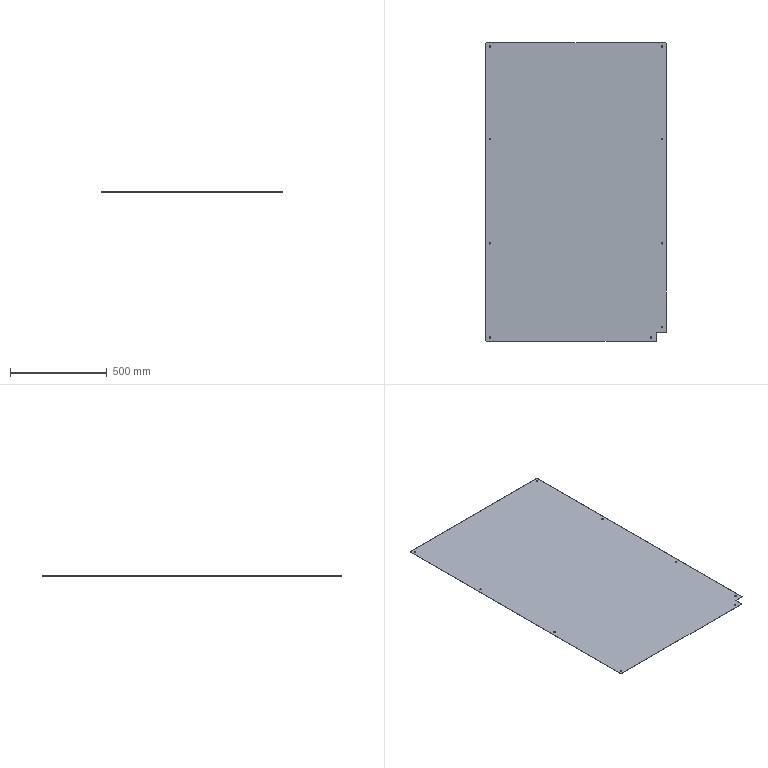Part | SolidWorks | features ICE 5, Fillet 2, FlatPattern 1, HoleWzd 1, SMBaseFlange 1, SheetMetal 1 | 1 solid | 32 faces | box 933 x 1548 x 1.2 mm | volume 1730124 mm3 | cylinder 24 | plane 8 | commonest cylinder face diameters 7 x18 6 x6
STEP:
#1=CARTESIAN_POINT('',(16.5,-20.,0.));
#2=VERTEX_POINT('',#1);
#3=CARTESIAN_POINT('',(23.5,-20.,0.));
#4=VERTEX_POINT('',#3);
#5=CARTESIAN_POINT('',(20.,-20.,0.));
#6=DIRECTION('',(0.,0.,1.));
#7=DIRECTION('',(1.,0.,0.));
#8=AXIS2_PLACEMENT_3D('',#5,#6,#7);
#9=CIRCLE('',#8,3.5);
#10=EDGE_CURVE('',#2,#4,#9,.T.);
#11=ORIENTED_EDGE('',*,*,#10,.F.);
#12=CARTESIAN_POINT('',(16.5,-20.,1.2));
#13=VERTEX_POINT('',#12);
#14=CARTESIAN_POINT('',(16.5,-20.,1.2));
#15=DIRECTION('',(0.,0.,1.));
#16=VECTOR('',#15,1000.);
#17=LINE('',#14,#16);
#18=EDGE_CURVE('',#2,#13,#17,.T.);
#19=ORIENTED_EDGE('',*,*,#18,.T.);
#20=CARTESIAN_POINT('',(23.5,-20.,1.2));
#21=VERTEX_POINT('',#20);
#22=CARTESIAN_POINT('',(20.,-20.,1.2));
#23=DIRECTION('',(0.,0.,1.));
#24=DIRECTION('',(1.,0.,0.));
#25=AXIS2_PLACEMENT_3D('',#22,#23,#24);
#26=CIRCLE('',#25,3.5);
#27=EDGE_CURVE('',#13,#21,#26,.T.);
#28=ORIENTED_EDGE('',*,*,#27,.T.);
#29=CARTESIAN_POINT('',(23.5,-20.,1.2));
#30=DIRECTION('',(0.,0.,1.));
#31=VECTOR('',#30,1000.);
#32=LINE('',#29,#31);
#33=EDGE_CURVE('',#4,#21,#32,.T.);
#34=ORIENTED_EDGE('',*,*,#33,.F.);
#35=EDGE_LOOP('',(#11,#19,#28,#34));
#36=FACE_OUTER_BOUND('',#35,.T.);
#37=CARTESIAN_POINT('',(20.,-20.,1.2));
#38=DIRECTION('',(0.,0.,1.));
#39=DIRECTION('',(1.,0.,0.));
#40=AXIS2_PLACEMENT_3D('',#37,#38,#39);
#41=CYLINDRICAL_SURFACE('',#40,3.5);
#42=ADVANCED_FACE('',(#36),#41,.F.);
#43=CARTESIAN_POINT('',(909.5,-20.,0.));
#44=VERTEX_POINT('',#43);
#45=CARTESIAN_POINT('',(916.5,-20.,0.));
#46=VERTEX_POINT('',#45);
#47=CARTESIAN_POINT('',(913.,-20.,0.));
#48=DIRECTION('',(0.,0.,1.));
#49=DIRECTION('',(1.,0.,0.));
#50=AXIS2_PLACEMENT_3D('',#47,#48,#49);
#51=CIRCLE('',#50,3.5);
#52=EDGE_CURVE('',#44,#46,#51,.T.);
#53=ORIENTED_EDGE('',*,*,#52,.F.);
#54=CARTESIAN_POINT('',(909.5,-20.,1.2));
#55=VERTEX_POINT('',#54);
#56=CARTESIAN_POINT('',(909.5,-20.,1.2));
#57=DIRECTION('',(0.,0.,1.));
#58=VECTOR('',#57,1000.);
#59=LINE('',#56,#58);
#60=EDGE_CURVE('',#44,#55,#59,.T.);
#61=ORIENTED_EDGE('',*,*,#60,.T.);
#62=CARTESIAN_POINT('',(916.5,-20.,1.2));
#63=VERTEX_POINT('',#62);
#64=CARTESIAN_POINT('',(913.,-20.,1.2));
#65=DIRECTION('',(0.,0.,1.));
#66=DIRECTION('',(1.,0.,0.));
#67=AXIS2_PLACEMENT_3D('',#64,#65,#66);
#68=CIRCLE('',#67,3.5);
#69=EDGE_CURVE('',#55,#63,#68,.T.);
#70=ORIENTED_EDGE('',*,*,#69,.T.);
#71=CARTESIAN_POINT('',(916.5,-20.,1.2));
#72=DIRECTION('',(0.,0.,1.));
#73=VECTOR('',#72,1000.);
#74=LINE('',#71,#73);
#75=EDGE_CURVE('',#46,#63,#74,.T.);
#76=ORIENTED_EDGE('',*,*,#75,.F.);
#77=EDGE_LOOP('',(#53,#61,#70,#76));
#78=FACE_OUTER_BOUND('',#77,.T.);
#79=CARTESIAN_POINT('',(913.,-20.,1.2));
#80=DIRECTION('',(0.,0.,1.));
#81=DIRECTION('',(1.,0.,0.));
#82=AXIS2_PLACEMENT_3D('',#79,#80,#81);
#83=CYLINDRICAL_SURFACE('',#82,3.5);
#84=ADVANCED_FACE('',(#78),#83,.F.);
#85=CARTESIAN_POINT('',(16.5,-1528.,0.));
#86=VERTEX_POINT('',#85);
#87=CARTESIAN_POINT('',(23.5,-1528.,0.));
#88=VERTEX_POINT('',#87);
#89=CARTESIAN_POINT('',(20.,-1528.,0.));
#90=DIRECTION('',(0.,0.,1.));
#91=DIRECTION('',(1.,0.,0.));
#92=AXIS2_PLACEMENT_3D('',#89,#90,#91);
#93=CIRCLE('',#92,3.5);
#94=EDGE_CURVE('',#86,#88,#93,.T.);
#95=ORIENTED_EDGE('',*,*,#94,.F.);
#96=CARTESIAN_POINT('',(16.5,-1528.,1.2));
#97=VERTEX_POINT('',#96);
#98=CARTESIAN_POINT('',(16.5,-1528.,1.2));
#99=DIRECTION('',(0.,0.,1.));
#100=VECTOR('',#99,1000.);
#101=LINE('',#98,#100);
#102=EDGE_CURVE('',#86,#97,#101,.T.);
#103=ORIENTED_EDGE('',*,*,#102,.T.);
#104=CARTESIAN_POINT('',(23.5,-1528.,1.2));
#105=VERTEX_POINT('',#104);
#106=CARTESIAN_POINT('',(20.,-1528.,1.2));
#107=DIRECTION('',(0.,0.,1.));
#108=DIRECTION('',(1.,0.,0.));
#109=AXIS2_PLACEMENT_3D('',#106,#107,#108);
#110=CIRCLE('',#109,3.5);
#111=EDGE_CURVE('',#97,#105,#110,.T.);
#112=ORIENTED_EDGE('',*,*,#111,.T.);
#113=CARTESIAN_POINT('',(23.5,-1528.,1.2));
#114=DIRECTION('',(0.,0.,1.));
#115=VECTOR('',#114,1000.);
#116=LINE('',#113,#115);
#117=EDGE_CURVE('',#88,#105,#116,.T.);
#118=ORIENTED_EDGE('',*,*,#117,.F.);
#119=EDGE_LOOP('',(#95,#103,#112,#118));
#120=FACE_OUTER_BOUND('',#119,.T.);
#121=CARTESIAN_POINT('',(20.,-1528.,1.2));
#122=DIRECTION('',(0.,0.,1.));
#123=DIRECTION('',(1.,0.,0.));
#124=AXIS2_PLACEMENT_3D('',#121,#122,#123);
#125=CYLINDRICAL_SURFACE('',#124,3.5);
#126=ADVANCED_FACE('',(#120),#125,.F.);
#127=CARTESIAN_POINT('',(851.5,-1528.,0.));
#128=VERTEX_POINT('',#127);
#129=CARTESIAN_POINT('',(858.5,-1528.,0.));
#130=VERTEX_POINT('',#129);
#131=CARTESIAN_POINT('',(855.,-1528.,0.));
#132=DIRECTION('',(0.,0.,1.));
#133=DIRECTION('',(1.,0.,0.));
#134=AXIS2_PLACEMENT_3D('',#131,#132,#133);
#135=CIRCLE('',#134,3.5);
#136=EDGE_CURVE('',#128,#130,#135,.T.);
#137=ORIENTED_EDGE('',*,*,#136,.F.);
#138=CARTESIAN_POINT('',(851.5,-1528.,1.2));
#139=VERTEX_POINT('',#138);
#140=CARTESIAN_POINT('',(851.5,-1528.,1.2));
#141=DIRECTION('',(0.,0.,1.));
#142=VECTOR('',#141,1000.);
#143=LINE('',#140,#142);
#144=EDGE_CURVE('',#128,#139,#143,.T.);
#145=ORIENTED_EDGE('',*,*,#144,.T.);
#146=CARTESIAN_POINT('',(858.5,-1528.,1.2));
#147=VERTEX_POINT('',#146);
#148=CARTESIAN_POINT('',(855.,-1528.,1.2));
#149=DIRECTION('',(0.,0.,1.));
#150=DIRECTION('',(1.,0.,0.));
#151=AXIS2_PLACEMENT_3D('',#148,#149,#150);
#152=CIRCLE('',#151,3.5);
#153=EDGE_CURVE('',#139,#147,#152,.T.);
#154=ORIENTED_EDGE('',*,*,#153,.T.);
#155=CARTESIAN_POINT('',(858.5,-1528.,1.2));
#156=DIRECTION('',(0.,0.,1.));
#157=VECTOR('',#156,1000.);
#158=LINE('',#155,#157);
#159=EDGE_CURVE('',#130,#147,#158,.T.);
#160=ORIENTED_EDGE('',*,*,#159,.F.);
#161=EDGE_LOOP('',(#137,#145,#154,#160));
#162=FACE_OUTER_BOUND('',#161,.T.);
#163=CARTESIAN_POINT('',(855.,-1528.,1.2));
#164=DIRECTION('',(0.,0.,1.));
#165=DIRECTION('',(1.,0.,0.));
#166=AXIS2_PLACEMENT_3D('',#163,#164,#165);
#167=CYLINDRICAL_SURFACE('',#166,3.5);
#168=ADVANCED_FACE('',(#162),#167,.F.);
#169=CARTESIAN_POINT('',(16.5,-1040.,0.));
#170=VERTEX_POINT('',#169);
#171=CARTESIAN_POINT('',(23.5,-1040.,0.));
#172=VERTEX_POINT('',#171);
#173=CARTESIAN_POINT('',(20.,-1040.,0.));
#174=DIRECTION('',(0.,0.,1.));
#175=DIRECTION('',(1.,0.,0.));
#176=AXIS2_PLACEMENT_3D('',#173,#174,#175);
#177=CIRCLE('',#176,3.5);
#178=EDGE_CURVE('',#170,#172,#177,.T.);
#179=ORIENTED_EDGE('',*,*,#178,.F.);
#180=CARTESIAN_POINT('',(16.5,-1040.,1.2));
#181=VERTEX_POINT('',#180);
#182=CARTESIAN_POINT('',(16.5,-1040.,1.2));
#183=DIRECTION('',(0.,0.,1.));
#184=VECTOR('',#183,1000.);
#185=LINE('',#182,#184);
#186=EDGE_CURVE('',#170,#181,#185,.T.);
#187=ORIENTED_EDGE('',*,*,#186,.T.);
#188=CARTESIAN_POINT('',(23.5,-1040.,1.2));
#189=VERTEX_POINT('',#188);
#190=CARTESIAN_POINT('',(20.,-1040.,1.2));
#191=DIRECTION('',(0.,0.,1.));
#192=DIRECTION('',(1.,0.,0.));
#193=AXIS2_PLACEMENT_3D('',#190,#191,#192);
#194=CIRCLE('',#193,3.5);
#195=EDGE_CURVE('',#181,#189,#194,.T.);
#196=ORIENTED_EDGE('',*,*,#195,.T.);
#197=CARTESIAN_POINT('',(23.5,-1040.,1.2));
#198=DIRECTION('',(0.,0.,1.));
#199=VECTOR('',#198,1000.);
#200=LINE('',#197,#199);
#201=EDGE_CURVE('',#172,#189,#200,.T.);
#202=ORIENTED_EDGE('',*,*,#201,.F.);
#203=EDGE_LOOP('',(#179,#187,#196,#202));
#204=FACE_OUTER_BOUND('',#203,.T.);
#205=CARTESIAN_POINT('',(20.,-1040.,1.2));
#206=DIRECTION('',(0.,0.,1.));
#207=DIRECTION('',(1.,0.,0.));
#208=AXIS2_PLACEMENT_3D('',#205,#206,#207);
#209=CYLINDRICAL_SURFACE('',#208,3.5);
#210=ADVANCED_FACE('',(#204),#209,.F.);
#211=CARTESIAN_POINT('',(909.5,-1040.,0.));
#212=VERTEX_POINT('',#211);
#213=CARTESIAN_POINT('',(916.5,-1040.,0.));
#214=VERTEX_POINT('',#213);
#215=CARTESIAN_POINT('',(913.,-1040.,0.));
#216=DIRECTION('',(0.,0.,1.));
#217=DIRECTION('',(1.,0.,0.));
#218=AXIS2_PLACEMENT_3D('',#215,#216,#217);
#219=CIRCLE('',#218,3.5);
#220=EDGE_CURVE('',#212,#214,#219,.T.);
#221=ORIENTED_EDGE('',*,*,#220,.F.);
#222=CARTESIAN_POINT('',(909.5,-1040.,1.2));
#223=VERTEX_POINT('',#222);
#224=CARTESIAN_POINT('',(909.5,-1040.,1.2));
#225=DIRECTION('',(0.,0.,1.));
#226=VECTOR('',#225,1000.);
#227=LINE('',#224,#226);
#228=EDGE_CURVE('',#212,#223,#227,.T.);
#229=ORIENTED_EDGE('',*,*,#228,.T.);
#230=CARTESIAN_POINT('',(916.5,-1040.,1.2));
#231=VERTEX_POINT('',#230);
#232=CARTESIAN_POINT('',(913.,-1040.,1.2));
#233=DIRECTION('',(0.,0.,1.));
#234=DIRECTION('',(1.,0.,0.));
#235=AXIS2_PLACEMENT_3D('',#232,#233,#234);
#236=CIRCLE('',#235,3.5);
#237=EDGE_CURVE('',#223,#231,#236,.T.);
#238=ORIENTED_EDGE('',*,*,#237,.T.);
#239=CARTESIAN_POINT('',(916.5,-1040.,1.2));
#240=DIRECTION('',(0.,0.,1.));
#241=VECTOR('',#240,1000.);
#242=LINE('',#239,#241);
#243=EDGE_CURVE('',#214,#231,#242,.T.);
#244=ORIENTED_EDGE('',*,*,#243,.F.);
#245=EDGE_LOOP('',(#221,#229,#238,#244));
#246=FACE_OUTER_BOUND('',#245,.T.);
#247=CARTESIAN_POINT('',(913.,-1040.,1.2));
#248=DIRECTION('',(0.,0.,1.));
#249=DIRECTION('',(1.,0.,0.));
#250=AXIS2_PLACEMENT_3D('',#247,#248,#249);
#251=CYLINDRICAL_SURFACE('',#250,3.5);
#252=ADVANCED_FACE('',(#246),#251,.F.);
#253=CARTESIAN_POINT('',(909.5,-1473.,0.));
#254=VERTEX_POINT('',#253);
#255=CARTESIAN_POINT('',(916.5,-1473.,0.));
#256=VERTEX_POINT('',#255);
#257=CARTESIAN_POINT('',(913.,-1473.,0.));
#258=DIRECTION('',(0.,0.,1.));
#259=DIRECTION('',(1.,0.,0.));
#260=AXIS2_PLACEMENT_3D('',#257,#258,#259);
#261=CIRCLE('',#260,3.5);
#262=EDGE_CURVE('',#254,#256,#261,.T.);
#263=ORIENTED_EDGE('',*,*,#262,.F.);
#264=CARTESIAN_POINT('',(909.5,-1473.,1.2));
#265=VERTEX_POINT('',#264);
#266=CARTESIAN_POINT('',(909.5,-1473.,1.2));
#267=DIRECTION('',(0.,0.,1.));
#268=VECTOR('',#267,1000.);
#269=LINE('',#266,#268);
#270=EDGE_CURVE('',#254,#265,#269,.T.);
#271=ORIENTED_EDGE('',*,*,#270,.T.);
#272=CARTESIAN_POINT('',(916.5,-1473.,1.2));
#273=VERTEX_POINT('',#272);
#274=CARTESIAN_POINT('',(913.,-1473.,1.2));
#275=DIRECTION('',(0.,0.,1.));
#276=DIRECTION('',(1.,0.,0.));
#277=AXIS2_PLACEMENT_3D('',#274,#275,#276);
#278=CIRCLE('',#277,3.5);
#279=EDGE_CURVE('',#265,#273,#278,.T.);
#280=ORIENTED_EDGE('',*,*,#279,.T.);
#281=CARTESIAN_POINT('',(916.5,-1473.,1.2));
#282=DIRECTION('',(0.,0.,1.));
#283=VECTOR('',#282,1000.);
#284=LINE('',#281,#283);
#285=EDGE_CURVE('',#256,#273,#284,.T.);
#286=ORIENTED_EDGE('',*,*,#285,.F.);
#287=EDGE_LOOP('',(#263,#271,#280,#286));
#288=FACE_OUTER_BOUND('',#287,.T.);
#289=CARTESIAN_POINT('',(913.,-1473.,1.2));
#290=DIRECTION('',(0.,0.,1.));
#291=DIRECTION('',(1.,0.,0.));
#292=AXIS2_PLACEMENT_3D('',#289,#290,#291);
#293=CYLINDRICAL_SURFACE('',#292,3.5);
#294=ADVANCED_FACE('',(#288),#293,.F.);
#295=CARTESIAN_POINT('',(16.5,-498.,0.));
#296=VERTEX_POINT('',#295);
#297=CARTESIAN_POINT('',(23.5,-498.,0.));
#298=VERTEX_POINT('',#297);
#299=CARTESIAN_POINT('',(20.,-498.,0.));
#300=DIRECTION('',(0.,0.,1.));
#301=DIRECTION('',(1.,0.,0.));
#302=AXIS2_PLACEMENT_3D('',#299,#300,#301);
#303=CIRCLE('',#302,3.5);
#304=EDGE_CURVE('',#296,#298,#303,.T.);
#305=ORIENTED_EDGE('',*,*,#304,.F.);
#306=CARTESIAN_POINT('',(16.5,-498.,1.2));
#307=VERTEX_POINT('',#306);
#308=CARTESIAN_POINT('',(16.5,-498.,1.2));
#309=DIRECTION('',(0.,0.,1.));
#310=VECTOR('',#309,1000.);
#311=LINE('',#308,#310);
#312=EDGE_CURVE('',#296,#307,#311,.T.);
#313=ORIENTED_EDGE('',*,*,#312,.T.);
#314=CARTESIAN_POINT('',(23.5,-498.,1.2));
#315=VERTEX_POINT('',#314);
#316=CARTESIAN_POINT('',(20.,-498.,1.2));
#317=DIRECTION('',(0.,0.,1.));
#318=DIRECTION('',(1.,0.,0.));
#319=AXIS2_PLACEMENT_3D('',#316,#317,#318);
#320=CIRCLE('',#319,3.5);
#321=EDGE_CURVE('',#307,#315,#320,.T.);
#322=ORIENTED_EDGE('',*,*,#321,.T.);
#323=CARTESIAN_POINT('',(23.5,-498.,1.2));
#324=DIRECTION('',(0.,0.,1.));
#325=VECTOR('',#324,1000.);
#326=LINE('',#323,#325);
#327=EDGE_CURVE('',#298,#315,#326,.T.);
#328=ORIENTED_EDGE('',*,*,#327,.F.);
#329=EDGE_LOOP('',(#305,#313,#322,#328));
#330=FACE_OUTER_BOUND('',#329,.T.);
#331=CARTESIAN_POINT('',(20.,-498.,1.2));
#332=DIRECTION('',(0.,0.,1.));
#333=DIRECTION('',(1.,0.,0.));
#334=AXIS2_PLACEMENT_3D('',#331,#332,#333);
#335=CYLINDRICAL_SURFACE('',#334,3.5);
#336=ADVANCED_FACE('',(#330),#335,.F.);
#337=CARTESIAN_POINT('',(909.5,-498.,0.));
#338=VERTEX_POINT('',#337);
#339=CARTESIAN_POINT('',(916.5,-498.,0.));
#340=VERTEX_POINT('',#339);
#341=CARTESIAN_POINT('',(913.,-498.,0.));
#342=DIRECTION('',(0.,0.,1.));
#343=DIRECTION('',(1.,0.,0.));
#344=AXIS2_PLACEMENT_3D('',#341,#342,#343);
#345=CIRCLE('',#344,3.5);
#346=EDGE_CURVE('',#338,#340,#345,.T.);
#347=ORIENTED_EDGE('',*,*,#346,.F.);
#348=CARTESIAN_POINT('',(909.5,-498.,1.2));
#349=VERTEX_POINT('',#348);
#350=CARTESIAN_POINT('',(909.5,-498.,1.2));
#351=DIRECTION('',(0.,0.,1.));
#352=VECTOR('',#351,1000.);
#353=LINE('',#350,#352);
#354=EDGE_CURVE('',#338,#349,#353,.T.);
#355=ORIENTED_EDGE('',*,*,#354,.T.);
#356=CARTESIAN_POINT('',(916.5,-498.,1.2));
#357=VERTEX_POINT('',#356);
#358=CARTESIAN_POINT('',(913.,-498.,1.2));
#359=DIRECTION('',(0.,0.,1.));
#360=DIRECTION('',(1.,0.,0.));
#361=AXIS2_PLACEMENT_3D('',#358,#359,#360);
#362=CIRCLE('',#361,3.5);
#363=EDGE_CURVE('',#349,#357,#362,.T.);
#364=ORIENTED_EDGE('',*,*,#363,.T.);
#365=CARTESIAN_POINT('',(916.5,-498.,1.2));
#366=DIRECTION('',(0.,0.,1.));
#367=VECTOR('',#366,1000.);
#368=LINE('',#365,#367);
#369=EDGE_CURVE('',#340,#357,#368,.T.);
#370=ORIENTED_EDGE('',*,*,#369,.F.);
#371=EDGE_LOOP('',(#347,#355,#364,#370));
#372=FACE_OUTER_BOUND('',#371,.T.);
#373=CARTESIAN_POINT('',(913.,-498.,1.2));
#374=DIRECTION('',(0.,0.,1.));
#375=DIRECTION('',(1.,0.,0.));
#376=AXIS2_PLACEMENT_3D('',#373,#374,#375);
#377=CYLINDRICAL_SURFACE('',#376,3.5);
#378=ADVANCED_FACE('',(#372),#377,.F.);
#379=CARTESIAN_POINT('',(3.,0.,1.2));
#380=VERTEX_POINT('',#379);
#381=CARTESIAN_POINT('',(930.,0.,1.2));
#382=VERTEX_POINT('',#381);
#383=CARTESIAN_POINT('',(0.,0.,1.2));
#384=DIRECTION('',(1.,0.,0.));
#385=VECTOR('',#384,1000.);
#386=LINE('',#383,#385);
#387=EDGE_CURVE('',#380,#382,#386,.T.);
#388=ORIENTED_EDGE('',*,*,#387,.T.);
#389=CARTESIAN_POINT('',(930.,0.,0.));
#390=VERTEX_POINT('',#389);
#391=CARTESIAN_POINT('',(930.,0.,0.));
#392=DIRECTION('',(0.,0.,-1.));
#393=VECTOR('',#392,1000.);
#394=LINE('',#391,#393);
#395=EDGE_CURVE('',#382,#390,#394,.T.);
#396=ORIENTED_EDGE('',*,*,#395,.T.);
#397=CARTESIAN_POINT('',(3.,0.,0.));
#398=VERTEX_POINT('',#397);
#399=CARTESIAN_POINT('',(0.,0.,0.));
#400=DIRECTION('',(1.,0.,0.));
#401=VECTOR('',#400,1000.);
#402=LINE('',#399,#401);
#403=EDGE_CURVE('',#398,#390,#402,.T.);
#404=ORIENTED_EDGE('',*,*,#403,.F.);
#405=CARTESIAN_POINT('',(3.,0.,1.2));
#406=DIRECTION('',(0.,0.,1.));
#407=VECTOR('',#406,1000.);
#408=LINE('',#405,#407);
#409=EDGE_CURVE('',#398,#380,#408,.T.);
#410=ORIENTED_EDGE('',*,*,#409,.T.);
#411=EDGE_LOOP('',(#388,#396,#404,#410));
#412=FACE_OUTER_BOUND('',#411,.T.);
#413=CARTESIAN_POINT('',(0.,0.,1.2));
#414=DIRECTION('',(0.,1.,0.));
#415=DIRECTION('',(0.,0.,1.));
#416=AXIS2_PLACEMENT_3D('',#413,#414,#415);
#417=PLANE('',#416);
#418=ADVANCED_FACE('',(#412),#417,.T.);
#419=CARTESIAN_POINT('',(20.,-20.,1.2));
#420=DIRECTION('',(0.,0.,1.));
#421=DIRECTION('',(1.,0.,0.));
#422=AXIS2_PLACEMENT_3D('',#419,#420,#421);
#423=CIRCLE('',#422,3.5);
#424=EDGE_CURVE('',#21,#13,#423,.T.);
#425=ORIENTED_EDGE('',*,*,#424,.F.);
#426=ORIENTED_EDGE('',*,*,#27,.F.);
#427=EDGE_LOOP('',(#425,#426));
#428=FACE_BOUND('',#427,.T.);
#429=CARTESIAN_POINT('',(913.,-20.,1.2));
#430=DIRECTION('',(0.,0.,1.));
#431=DIRECTION('',(1.,0.,0.));
#432=AXIS2_PLACEMENT_3D('',#429,#430,#431);
#433=CIRCLE('',#432,3.5);
#434=EDGE_CURVE('',#63,#55,#433,.T.);
#435=ORIENTED_EDGE('',*,*,#434,.F.);
#436=ORIENTED_EDGE('',*,*,#69,.F.);
#437=EDGE_LOOP('',(#435,#436));
#438=FACE_BOUND('',#437,.T.);
#439=CARTESIAN_POINT('',(20.,-1528.,1.2));
#440=DIRECTION('',(0.,0.,1.));
#441=DIRECTION('',(1.,0.,0.));
#442=AXIS2_PLACEMENT_3D('',#439,#440,#441);
#443=CIRCLE('',#442,3.5);
#444=EDGE_CURVE('',#105,#97,#443,.T.);
#445=ORIENTED_EDGE('',*,*,#444,.F.);
#446=ORIENTED_EDGE('',*,*,#111,.F.);
#447=EDGE_LOOP('',(#445,#446));
#448=FACE_BOUND('',#447,.T.);
#449=CARTESIAN_POINT('',(855.,-1528.,1.2));
#450=DIRECTION('',(0.,0.,1.));
#451=DIRECTION('',(1.,0.,0.));
#452=AXIS2_PLACEMENT_3D('',#449,#450,#451);
#453=CIRCLE('',#452,3.5);
#454=EDGE_CURVE('',#147,#139,#453,.T.);
#455=ORIENTED_EDGE('',*,*,#454,.F.);
#456=ORIENTED_EDGE('',*,*,#153,.F.);
#457=EDGE_LOOP('',(#455,#456));
#458=FACE_BOUND('',#457,.T.);
#459=CARTESIAN_POINT('',(20.,-1040.,1.2));
#460=DIRECTION('',(0.,0.,1.));
#461=DIRECTION('',(1.,0.,0.));
#462=AXIS2_PLACEMENT_3D('',#459,#460,#461);
#463=CIRCLE('',#462,3.5);
#464=EDGE_CURVE('',#189,#181,#463,.T.);
#465=ORIENTED_EDGE('',*,*,#464,.F.);
#466=ORIENTED_EDGE('',*,*,#195,.F.);
#467=EDGE_LOOP('',(#465,#466));
#468=FACE_BOUND('',#467,.T.);
#469=CARTESIAN_POINT('',(913.,-1040.,1.2));
#470=DIRECTION('',(0.,0.,1.));
#471=DIRECTION('',(1.,0.,0.));
#472=AXIS2_PLACEMENT_3D('',#469,#470,#471);
#473=CIRCLE('',#472,3.5);
#474=EDGE_CURVE('',#231,#223,#473,.T.);
#475=ORIENTED_EDGE('',*,*,#474,.F.);
#476=ORIENTED_EDGE('',*,*,#237,.F.);
#477=EDGE_LOOP('',(#475,#476));
#478=FACE_BOUND('',#477,.T.);
#479=CARTESIAN_POINT('',(913.,-1473.,1.2));
#480=DIRECTION('',(0.,0.,1.));
#481=DIRECTION('',(1.,0.,0.));
#482=AXIS2_PLACEMENT_3D('',#479,#480,#481);
#483=CIRCLE('',#482,3.5);
#484=EDGE_CURVE('',#273,#265,#483,.T.);
#485=ORIENTED_EDGE('',*,*,#484,.F.);
#486=ORIENTED_EDGE('',*,*,#279,.F.);
#487=EDGE_LOOP('',(#485,#486));
#488=FACE_BOUND('',#487,.T.);
#489=CARTESIAN_POINT('',(20.,-498.,1.2));
#490=DIRECTION('',(0.,0.,1.));
#491=DIRECTION('',(1.,0.,0.));
#492=AXIS2_PLACEMENT_3D('',#489,#490,#491);
#493=CIRCLE('',#492,3.5);
#494=EDGE_CURVE('',#315,#307,#493,.T.);
#495=ORIENTED_EDGE('',*,*,#494,.F.);
#496=ORIENTED_EDGE('',*,*,#321,.F.);
#497=EDGE_LOOP('',(#495,#496));
#498=FACE_BOUND('',#497,.T.);
#499=CARTESIAN_POINT('',(913.,-498.,1.2));
#500=DIRECTION('',(0.,0.,1.));
#501=DIRECTION('',(1.,0.,0.));
#502=AXIS2_PLACEMENT_3D('',#499,#500,#501);
#503=CIRCLE('',#502,3.5);
#504=EDGE_CURVE('',#357,#349,#503,.T.);
#505=ORIENTED_EDGE('',*,*,#504,.F.);
#506=ORIENTED_EDGE('',*,*,#363,.F.);
#507=EDGE_LOOP('',(#505,#506));
#508=FACE_BOUND('',#507,.T.);
#509=CARTESIAN_POINT('',(930.,-1503.,1.2));
#510=VERTEX_POINT('',#509);
#511=CARTESIAN_POINT('',(888.,-1503.,1.2));
#512=VERTEX_POINT('',#511);
#513=CARTESIAN_POINT('',(885.,-1503.,1.2));
#514=DIRECTION('',(-1.,0.,0.));
#515=VECTOR('',#514,1000.);
#516=LINE('',#513,#515);
#517=EDGE_CURVE('',#510,#512,#516,.T.);
#518=ORIENTED_EDGE('',*,*,#517,.F.);
#519=CARTESIAN_POINT('',(933.,-1500.,1.2));
#520=VERTEX_POINT('',#519);
#521=CARTESIAN_POINT('',(930.,-1500.,1.2));
#522=DIRECTION('',(0.,0.,1.));
#523=DIRECTION('',(1.,0.,0.));
#524=AXIS2_PLACEMENT_3D('',#521,#522,#523);
#525=CIRCLE('',#524,3.);
#526=EDGE_CURVE('',#510,#520,#525,.T.);
#527=ORIENTED_EDGE('',*,*,#526,.T.);
#528=CARTESIAN_POINT('',(933.,-3.,1.2));
#529=VERTEX_POINT('',#528);
#530=CARTESIAN_POINT('',(933.,-1651.39,1.2));
#531=DIRECTION('',(0.,-1.,0.));
#532=VECTOR('',#531,1000.);
#533=LINE('',#530,#532);
#534=EDGE_CURVE('',#529,#520,#533,.T.);
#535=ORIENTED_EDGE('',*,*,#534,.F.);
#536=CARTESIAN_POINT('',(930.,-3.,1.2));
#537=DIRECTION('',(0.,0.,1.));
#538=DIRECTION('',(1.,0.,0.));
#539=AXIS2_PLACEMENT_3D('',#536,#537,#538);
#540=CIRCLE('',#539,3.);
#541=EDGE_CURVE('',#529,#382,#540,.T.);
#542=ORIENTED_EDGE('',*,*,#541,.T.);
#543=ORIENTED_EDGE('',*,*,#387,.F.);
#544=CARTESIAN_POINT('',(0.,-3.,1.2));
#545=VERTEX_POINT('',#544);
#546=CARTESIAN_POINT('',(3.,-3.,1.2));
#547=DIRECTION('',(0.,0.,1.));
#548=DIRECTION('',(1.,0.,0.));
#549=AXIS2_PLACEMENT_3D('',#546,#547,#548);
#550=CIRCLE('',#549,3.);
#551=EDGE_CURVE('',#380,#545,#550,.T.);
#552=ORIENTED_EDGE('',*,*,#551,.T.);
#553=CARTESIAN_POINT('',(0.,-1545.,1.2));
#554=VERTEX_POINT('',#553);
#555=CARTESIAN_POINT('',(0.,0.,1.2));
#556=DIRECTION('',(0.,1.,0.));
#557=VECTOR('',#556,1000.);
#558=LINE('',#555,#557);
#559=EDGE_CURVE('',#554,#545,#558,.T.);
#560=ORIENTED_EDGE('',*,*,#559,.F.);
#561=CARTESIAN_POINT('',(3.,-1548.,1.2));
#562=VERTEX_POINT('',#561);
#563=CARTESIAN_POINT('',(3.,-1545.,1.2));
#564=DIRECTION('',(0.,0.,1.));
#565=DIRECTION('',(1.,0.,0.));
#566=AXIS2_PLACEMENT_3D('',#563,#564,#565);
#567=CIRCLE('',#566,3.);
#568=EDGE_CURVE('',#554,#562,#567,.T.);
#569=ORIENTED_EDGE('',*,*,#568,.T.);
#570=CARTESIAN_POINT('',(882.,-1548.,1.2));
#571=VERTEX_POINT('',#570);
#572=CARTESIAN_POINT('',(0.,-1548.,1.2));
#573=DIRECTION('',(-1.,0.,0.));
#574=VECTOR('',#573,1000.);
#575=LINE('',#572,#574);
#576=EDGE_CURVE('',#571,#562,#575,.T.);
#577=ORIENTED_EDGE('',*,*,#576,.F.);
#578=CARTESIAN_POINT('',(885.,-1545.,1.2));
#579=VERTEX_POINT('',#578);
#580=CARTESIAN_POINT('',(882.,-1545.,1.2));
#581=DIRECTION('',(0.,0.,1.));
#582=DIRECTION('',(1.,0.,0.));
#583=AXIS2_PLACEMENT_3D('',#580,#581,#582);
#584=CIRCLE('',#583,3.);
#585=EDGE_CURVE('',#571,#579,#584,.T.);
#586=ORIENTED_EDGE('',*,*,#585,.T.);
#587=CARTESIAN_POINT('',(885.,-1506.,1.2));
#588=VERTEX_POINT('',#587);
#589=CARTESIAN_POINT('',(885.,-1548.,1.2));
#590=DIRECTION('',(0.,-1.,0.));
#591=VECTOR('',#590,1000.);
#592=LINE('',#589,#591);
#593=EDGE_CURVE('',#588,#579,#592,.T.);
#594=ORIENTED_EDGE('',*,*,#593,.F.);
#595=CARTESIAN_POINT('',(888.,-1506.,1.2));
#596=DIRECTION('',(0.,0.,-1.));
#597=DIRECTION('',(1.,0.,0.));
#598=AXIS2_PLACEMENT_3D('',#595,#596,#597);
#599=CIRCLE('',#598,3.);
#600=EDGE_CURVE('',#588,#512,#599,.T.);
#601=ORIENTED_EDGE('',*,*,#600,.T.);
#602=EDGE_LOOP('',(#518,#527,#535,#542,#543,#552,#560,#569,#577,#586,#594,#601));
#603=FACE_OUTER_BOUND('',#602,.T.);
#604=CARTESIAN_POINT('',(0.,0.,1.2));
#605=DIRECTION('',(0.,0.,1.));
#606=DIRECTION('',(1.,0.,0.));
#607=AXIS2_PLACEMENT_3D('',#604,#605,#606);
#608=PLANE('',#607);
#609=ADVANCED_FACE('',(#428,#438,#448,#458,#468,#478,#488,#498,#508,#603),#608,.T.);
#610=CARTESIAN_POINT('',(20.,-20.,0.));
#611=DIRECTION('',(0.,0.,1.));
#612=DIRECTION('',(1.,0.,0.));
#613=AXIS2_PLACEMENT_3D('',#610,#611,#612);
#614=CIRCLE('',#613,3.5);
#615=EDGE_CURVE('',#4,#2,#614,.T.);
#616=ORIENTED_EDGE('',*,*,#615,.T.);
#617=ORIENTED_EDGE('',*,*,#10,.T.);
#618=EDGE_LOOP('',(#616,#617));
#619=FACE_BOUND('',#618,.T.);
#620=CARTESIAN_POINT('',(913.,-20.,0.));
#621=DIRECTION('',(0.,0.,1.));
#622=DIRECTION('',(1.,0.,0.));
#623=AXIS2_PLACEMENT_3D('',#620,#621,#622);
#624=CIRCLE('',#623,3.5);
#625=EDGE_CURVE('',#46,#44,#624,.T.);
#626=ORIENTED_EDGE('',*,*,#625,.T.);
#627=ORIENTED_EDGE('',*,*,#52,.T.);
#628=EDGE_LOOP('',(#626,#627));
#629=FACE_BOUND('',#628,.T.);
#630=CARTESIAN_POINT('',(20.,-1528.,0.));
#631=DIRECTION('',(0.,0.,1.));
#632=DIRECTION('',(1.,0.,0.));
#633=AXIS2_PLACEMENT_3D('',#630,#631,#632);
#634=CIRCLE('',#633,3.5);
#635=EDGE_CURVE('',#88,#86,#634,.T.);
#636=ORIENTED_EDGE('',*,*,#635,.T.);
#637=ORIENTED_EDGE('',*,*,#94,.T.);
#638=EDGE_LOOP('',(#636,#637));
#639=FACE_BOUND('',#638,.T.);
#640=CARTESIAN_POINT('',(855.,-1528.,0.));
#641=DIRECTION('',(0.,0.,1.));
#642=DIRECTION('',(1.,0.,0.));
#643=AXIS2_PLACEMENT_3D('',#640,#641,#642);
#644=CIRCLE('',#643,3.5);
#645=EDGE_CURVE('',#130,#128,#644,.T.);
#646=ORIENTED_EDGE('',*,*,#645,.T.);
#647=ORIENTED_EDGE('',*,*,#136,.T.);
#648=EDGE_LOOP('',(#646,#647));
#649=FACE_BOUND('',#648,.T.);
#650=CARTESIAN_POINT('',(20.,-1040.,0.));
#651=DIRECTION('',(0.,0.,1.));
#652=DIRECTION('',(1.,0.,0.));
#653=AXIS2_PLACEMENT_3D('',#650,#651,#652);
#654=CIRCLE('',#653,3.5);
#655=EDGE_CURVE('',#172,#170,#654,.T.);
#656=ORIENTED_EDGE('',*,*,#655,.T.);
#657=ORIENTED_EDGE('',*,*,#178,.T.);
#658=EDGE_LOOP('',(#656,#657));
#659=FACE_BOUND('',#658,.T.);
#660=CARTESIAN_POINT('',(913.,-1040.,0.));
#661=DIRECTION('',(0.,0.,1.));
#662=DIRECTION('',(1.,0.,0.));
#663=AXIS2_PLACEMENT_3D('',#660,#661,#662);
#664=CIRCLE('',#663,3.5);
#665=EDGE_CURVE('',#214,#212,#664,.T.);
#666=ORIENTED_EDGE('',*,*,#665,.T.);
#667=ORIENTED_EDGE('',*,*,#220,.T.);
#668=EDGE_LOOP('',(#666,#667));
#669=FACE_BOUND('',#668,.T.);
#670=CARTESIAN_POINT('',(913.,-1473.,0.));
#671=DIRECTION('',(0.,0.,1.));
#672=DIRECTION('',(1.,0.,0.));
#673=AXIS2_PLACEMENT_3D('',#670,#671,#672);
#674=CIRCLE('',#673,3.5);
#675=EDGE_CURVE('',#256,#254,#674,.T.);
#676=ORIENTED_EDGE('',*,*,#675,.T.);
#677=ORIENTED_EDGE('',*,*,#262,.T.);
#678=EDGE_LOOP('',(#676,#677));
#679=FACE_BOUND('',#678,.T.);
#680=CARTESIAN_POINT('',(20.,-498.,0.));
#681=DIRECTION('',(0.,0.,1.));
#682=DIRECTION('',(1.,0.,0.));
#683=AXIS2_PLACEMENT_3D('',#680,#681,#682);
#684=CIRCLE('',#683,3.5);
#685=EDGE_CURVE('',#298,#296,#684,.T.);
#686=ORIENTED_EDGE('',*,*,#685,.T.);
#687=ORIENTED_EDGE('',*,*,#304,.T.);
#688=EDGE_LOOP('',(#686,#687));
#689=FACE_BOUND('',#688,.T.);
#690=CARTESIAN_POINT('',(913.,-498.,0.));
#691=DIRECTION('',(0.,0.,1.));
#692=DIRECTION('',(1.,0.,0.));
#693=AXIS2_PLACEMENT_3D('',#690,#691,#692);
#694=CIRCLE('',#693,3.5);
#695=EDGE_CURVE('',#340,#338,#694,.T.);
#696=ORIENTED_EDGE('',*,*,#695,.T.);
#697=ORIENTED_EDGE('',*,*,#346,.T.);
#698=EDGE_LOOP('',(#696,#697));
#699=FACE_BOUND('',#698,.T.);
#700=CARTESIAN_POINT('',(933.,-3.,0.));
#701=VERTEX_POINT('',#700);
#702=CARTESIAN_POINT('',(933.,-1500.,0.));
#703=VERTEX_POINT('',#702);
#704=CARTESIAN_POINT('',(933.,0.,0.));
#705=DIRECTION('',(0.,-1.,0.));
#706=VECTOR('',#705,1000.);
#707=LINE('',#704,#706);
#708=EDGE_CURVE('',#701,#703,#707,.T.);
#709=ORIENTED_EDGE('',*,*,#708,.T.);
#710=CARTESIAN_POINT('',(930.,-1503.,0.));
#711=VERTEX_POINT('',#710);
#712=CARTESIAN_POINT('',(930.,-1500.,0.));
#713=DIRECTION('',(0.,0.,-1.));
#714=DIRECTION('',(1.,0.,0.));
#715=AXIS2_PLACEMENT_3D('',#712,#713,#714);
#716=CIRCLE('',#715,3.);
#717=EDGE_CURVE('',#703,#711,#716,.T.);
#718=ORIENTED_EDGE('',*,*,#717,.T.);
#719=CARTESIAN_POINT('',(888.,-1503.,0.));
#720=VERTEX_POINT('',#719);
#721=CARTESIAN_POINT('',(0.,-1503.,0.));
#722=DIRECTION('',(-1.,0.,0.));
#723=VECTOR('',#722,1000.);
#724=LINE('',#721,#723);
#725=EDGE_CURVE('',#711,#720,#724,.T.);
#726=ORIENTED_EDGE('',*,*,#725,.T.);
#727=CARTESIAN_POINT('',(885.,-1506.,0.));
#728=VERTEX_POINT('',#727);
#729=CARTESIAN_POINT('',(888.,-1506.,0.));
#730=DIRECTION('',(0.,0.,1.));
#731=DIRECTION('',(1.,0.,0.));
#732=AXIS2_PLACEMENT_3D('',#729,#730,#731);
#733=CIRCLE('',#732,3.);
#734=EDGE_CURVE('',#720,#728,#733,.T.);
#735=ORIENTED_EDGE('',*,*,#734,.T.);
#736=CARTESIAN_POINT('',(885.,-1545.,0.));
#737=VERTEX_POINT('',#736);
#738=CARTESIAN_POINT('',(885.,0.,0.));
#739=DIRECTION('',(0.,-1.,0.));
#740=VECTOR('',#739,1000.);
#741=LINE('',#738,#740);
#742=EDGE_CURVE('',#728,#737,#741,.T.);
#743=ORIENTED_EDGE('',*,*,#742,.T.);
#744=CARTESIAN_POINT('',(882.,-1548.,0.));
#745=VERTEX_POINT('',#744);
#746=CARTESIAN_POINT('',(882.,-1545.,0.));
#747=DIRECTION('',(0.,0.,-1.));
#748=DIRECTION('',(1.,0.,0.));
#749=AXIS2_PLACEMENT_3D('',#746,#747,#748);
#750=CIRCLE('',#749,3.);
#751=EDGE_CURVE('',#737,#745,#750,.T.);
#752=ORIENTED_EDGE('',*,*,#751,.T.);
#753=CARTESIAN_POINT('',(3.,-1548.,0.));
#754=VERTEX_POINT('',#753);
#755=CARTESIAN_POINT('',(0.,-1548.,0.));
#756=DIRECTION('',(-1.,0.,0.));
#757=VECTOR('',#756,1000.);
#758=LINE('',#755,#757);
#759=EDGE_CURVE('',#745,#754,#758,.T.);
#760=ORIENTED_EDGE('',*,*,#759,.T.);
#761=CARTESIAN_POINT('',(0.,-1545.,0.));
#762=VERTEX_POINT('',#761);
#763=CARTESIAN_POINT('',(3.,-1545.,0.));
#764=DIRECTION('',(0.,0.,-1.));
#765=DIRECTION('',(1.,0.,0.));
#766=AXIS2_PLACEMENT_3D('',#763,#764,#765);
#767=CIRCLE('',#766,3.);
#768=EDGE_CURVE('',#754,#762,#767,.T.);
#769=ORIENTED_EDGE('',*,*,#768,.T.);
#770=CARTESIAN_POINT('',(0.,-3.,0.));
#771=VERTEX_POINT('',#770);
#772=CARTESIAN_POINT('',(0.,0.,0.));
#773=DIRECTION('',(0.,1.,0.));
#774=VECTOR('',#773,1000.);
#775=LINE('',#772,#774);
#776=EDGE_CURVE('',#762,#771,#775,.T.);
#777=ORIENTED_EDGE('',*,*,#776,.T.);
#778=CARTESIAN_POINT('',(3.,-3.,0.));
#779=DIRECTION('',(0.,0.,-1.));
#780=DIRECTION('',(1.,0.,0.));
#781=AXIS2_PLACEMENT_3D('',#778,#779,#780);
#782=CIRCLE('',#781,3.);
#783=EDGE_CURVE('',#771,#398,#782,.T.);
#784=ORIENTED_EDGE('',*,*,#783,.T.);
#785=ORIENTED_EDGE('',*,*,#403,.T.);
#786=CARTESIAN_POINT('',(930.,-3.,0.));
#787=DIRECTION('',(0.,0.,-1.));
#788=DIRECTION('',(1.,0.,0.));
#789=AXIS2_PLACEMENT_3D('',#786,#787,#788);
#790=CIRCLE('',#789,3.);
#791=EDGE_CURVE('',#390,#701,#790,.T.);
#792=ORIENTED_EDGE('',*,*,#791,.T.);
#793=EDGE_LOOP('',(#709,#718,#726,#735,#743,#752,#760,#769,#777,#784,#785,#792));
#794=FACE_OUTER_BOUND('',#793,.T.);
#795=CARTESIAN_POINT('',(0.,0.,0.));
#796=DIRECTION('',(0.,0.,1.));
#797=DIRECTION('',(1.,0.,0.));
#798=AXIS2_PLACEMENT_3D('',#795,#796,#797);
#799=PLANE('',#798);
#800=ADVANCED_FACE('',(#619,#629,#639,#649,#659,#669,#679,#689,#699,#794),#799,.F.);
#801=ORIENTED_EDGE('',*,*,#725,.F.);
#802=CARTESIAN_POINT('',(930.,-1503.,-8.8));
#803=DIRECTION('',(0.,0.,1.));
#804=VECTOR('',#803,1000.);
#805=LINE('',#802,#804);
#806=EDGE_CURVE('',#711,#510,#805,.T.);
#807=ORIENTED_EDGE('',*,*,#806,.T.);
#808=ORIENTED_EDGE('',*,*,#517,.T.);
#809=CARTESIAN_POINT('',(888.,-1503.,0.));
#810=DIRECTION('',(0.,0.,-1.));
#811=VECTOR('',#810,1000.);
#812=LINE('',#809,#811);
#813=EDGE_CURVE('',#512,#720,#812,.T.);
#814=ORIENTED_EDGE('',*,*,#813,.T.);
#815=EDGE_LOOP('',(#801,#807,#808,#814));
#816=FACE_OUTER_BOUND('',#815,.T.);
#817=CARTESIAN_POINT('',(885.,-1503.,-8.8));
#818=DIRECTION('',(0.,1.,0.));
#819=DIRECTION('',(0.,0.,1.));
#820=AXIS2_PLACEMENT_3D('',#817,#818,#819);
#821=PLANE('',#820);
#822=ADVANCED_FACE('',(#816),#821,.F.);
#823=ORIENTED_EDGE('',*,*,#759,.F.);
#824=CARTESIAN_POINT('',(882.,-1548.,1.2));
#825=DIRECTION('',(0.,0.,1.));
#826=VECTOR('',#825,1000.);
#827=LINE('',#824,#826);
#828=EDGE_CURVE('',#745,#571,#827,.T.);
#829=ORIENTED_EDGE('',*,*,#828,.T.);
#830=ORIENTED_EDGE('',*,*,#576,.T.);
#831=CARTESIAN_POINT('',(3.,-1548.,1.2));
#832=DIRECTION('',(0.,0.,-1.));
#833=VECTOR('',#832,1000.);
#834=LINE('',#831,#833);
#835=EDGE_CURVE('',#562,#754,#834,.T.);
#836=ORIENTED_EDGE('',*,*,#835,.T.);
#837=EDGE_LOOP('',(#823,#829,#830,#836));
#838=FACE_OUTER_BOUND('',#837,.T.);
#839=CARTESIAN_POINT('',(0.,-1548.,1.2));
#840=DIRECTION('',(0.,-1.,0.));
#841=DIRECTION('',(0.,0.,-1.));
#842=AXIS2_PLACEMENT_3D('',#839,#840,#841);
#843=PLANE('',#842);
#844=ADVANCED_FACE('',(#838),#843,.T.);
#845=ORIENTED_EDGE('',*,*,#776,.F.);
#846=CARTESIAN_POINT('',(0.,-1545.,1.2));
#847=DIRECTION('',(0.,0.,1.));
#848=VECTOR('',#847,1000.);
#849=LINE('',#846,#848);
#850=EDGE_CURVE('',#762,#554,#849,.T.);
#851=ORIENTED_EDGE('',*,*,#850,.T.);
#852=ORIENTED_EDGE('',*,*,#559,.T.);
#853=CARTESIAN_POINT('',(0.,-3.,1.2));
#854=DIRECTION('',(0.,0.,-1.));
#855=VECTOR('',#854,1000.);
#856=LINE('',#853,#855);
#857=EDGE_CURVE('',#545,#771,#856,.T.);
#858=ORIENTED_EDGE('',*,*,#857,.T.);
#859=EDGE_LOOP('',(#845,#851,#852,#858));
#860=FACE_OUTER_BOUND('',#859,.T.);
#861=CARTESIAN_POINT('',(0.,0.,1.2));
#862=DIRECTION('',(-1.,0.,0.));
#863=DIRECTION('',(0.,0.,1.));
#864=AXIS2_PLACEMENT_3D('',#861,#862,#863);
#865=PLANE('',#864);
#866=ADVANCED_FACE('',(#860),#865,.T.);
#867=ORIENTED_EDGE('',*,*,#742,.F.);
#868=CARTESIAN_POINT('',(885.,-1506.,1.2));
#869=DIRECTION('',(0.,0.,1.));
#870=VECTOR('',#869,1000.);
#871=LINE('',#868,#870);
#872=EDGE_CURVE('',#728,#588,#871,.T.);
#873=ORIENTED_EDGE('',*,*,#872,.T.);
#874=ORIENTED_EDGE('',*,*,#593,.T.);
#875=CARTESIAN_POINT('',(885.,-1545.,0.));
#876=DIRECTION('',(0.,0.,-1.));
#877=VECTOR('',#876,1000.);
#878=LINE('',#875,#877);
#879=EDGE_CURVE('',#579,#737,#878,.T.);
#880=ORIENTED_EDGE('',*,*,#879,.T.);
#881=EDGE_LOOP('',(#867,#873,#874,#880));
#882=FACE_OUTER_BOUND('',#881,.T.);
#883=CARTESIAN_POINT('',(885.,-1548.,-8.8));
#884=DIRECTION('',(-1.,0.,0.));
#885=DIRECTION('',(0.,-1.,0.));
#886=AXIS2_PLACEMENT_3D('',#883,#884,#885);
#887=PLANE('',#886);
#888=ADVANCED_FACE('',(#882),#887,.F.);
#889=ORIENTED_EDGE('',*,*,#534,.T.);
#890=CARTESIAN_POINT('',(933.,-1500.,-8.8));
#891=DIRECTION('',(0.,0.,-1.));
#892=VECTOR('',#891,1000.);
#893=LINE('',#890,#892);
#894=EDGE_CURVE('',#520,#703,#893,.T.);
#895=ORIENTED_EDGE('',*,*,#894,.T.);
#896=ORIENTED_EDGE('',*,*,#708,.F.);
#897=CARTESIAN_POINT('',(933.,-3.,1.2));
#898=DIRECTION('',(0.,0.,1.));
#899=VECTOR('',#898,1000.);
#900=LINE('',#897,#899);
#901=EDGE_CURVE('',#701,#529,#900,.T.);
#902=ORIENTED_EDGE('',*,*,#901,.T.);
#903=EDGE_LOOP('',(#889,#895,#896,#902));
#904=FACE_OUTER_BOUND('',#903,.T.);
#905=CARTESIAN_POINT('',(933.,-1651.39,-8.8));
#906=DIRECTION('',(-1.,0.,0.));
#907=DIRECTION('',(0.,0.,1.));
#908=AXIS2_PLACEMENT_3D('',#905,#906,#907);
#909=PLANE('',#908);
#910=ADVANCED_FACE('',(#904),#909,.F.);
#911=ORIENTED_EDGE('',*,*,#354,.F.);
#912=ORIENTED_EDGE('',*,*,#695,.F.);
#913=ORIENTED_EDGE('',*,*,#369,.T.);
#914=ORIENTED_EDGE('',*,*,#504,.T.);
#915=EDGE_LOOP('',(#911,#912,#913,#914));
#916=FACE_OUTER_BOUND('',#915,.T.);
#917=CARTESIAN_POINT('',(913.,-498.,1.2));
#918=DIRECTION('',(0.,0.,1.));
#919=DIRECTION('',(1.,0.,0.));
#920=AXIS2_PLACEMENT_3D('',#917,#918,#919);
#921=CYLINDRICAL_SURFACE('',#920,3.5);
#922=ADVANCED_FACE('',(#916),#921,.F.);
#923=ORIENTED_EDGE('',*,*,#312,.F.);
#924=ORIENTED_EDGE('',*,*,#685,.F.);
#925=ORIENTED_EDGE('',*,*,#327,.T.);
#926=ORIENTED_EDGE('',*,*,#494,.T.);
#927=EDGE_LOOP('',(#923,#924,#925,#926));
#928=FACE_OUTER_BOUND('',#927,.T.);
#929=CARTESIAN_POINT('',(20.,-498.,1.2));
#930=DIRECTION('',(0.,0.,1.));
#931=DIRECTION('',(1.,0.,0.));
#932=AXIS2_PLACEMENT_3D('',#929,#930,#931);
#933=CYLINDRICAL_SURFACE('',#932,3.5);
#934=ADVANCED_FACE('',(#928),#933,.F.);
#935=ORIENTED_EDGE('',*,*,#270,.F.);
#936=ORIENTED_EDGE('',*,*,#675,.F.);
#937=ORIENTED_EDGE('',*,*,#285,.T.);
#938=ORIENTED_EDGE('',*,*,#484,.T.);
#939=EDGE_LOOP('',(#935,#936,#937,#938));
#940=FACE_OUTER_BOUND('',#939,.T.);
#941=CARTESIAN_POINT('',(913.,-1473.,1.2));
#942=DIRECTION('',(0.,0.,1.));
#943=DIRECTION('',(1.,0.,0.));
#944=AXIS2_PLACEMENT_3D('',#941,#942,#943);
#945=CYLINDRICAL_SURFACE('',#944,3.5);
#946=ADVANCED_FACE('',(#940),#945,.F.);
#947=ORIENTED_EDGE('',*,*,#228,.F.);
#948=ORIENTED_EDGE('',*,*,#665,.F.);
#949=ORIENTED_EDGE('',*,*,#243,.T.);
#950=ORIENTED_EDGE('',*,*,#474,.T.);
#951=EDGE_LOOP('',(#947,#948,#949,#950));
#952=FACE_OUTER_BOUND('',#951,.T.);
#953=CARTESIAN_POINT('',(913.,-1040.,1.2));
#954=DIRECTION('',(0.,0.,1.));
#955=DIRECTION('',(1.,0.,0.));
#956=AXIS2_PLACEMENT_3D('',#953,#954,#955);
#957=CYLINDRICAL_SURFACE('',#956,3.5);
#958=ADVANCED_FACE('',(#952),#957,.F.);
#959=ORIENTED_EDGE('',*,*,#186,.F.);
#960=ORIENTED_EDGE('',*,*,#655,.F.);
#961=ORIENTED_EDGE('',*,*,#201,.T.);
#962=ORIENTED_EDGE('',*,*,#464,.T.);
#963=EDGE_LOOP('',(#959,#960,#961,#962));
#964=FACE_OUTER_BOUND('',#963,.T.);
#965=CARTESIAN_POINT('',(20.,-1040.,1.2));
#966=DIRECTION('',(0.,0.,1.));
#967=DIRECTION('',(1.,0.,0.));
#968=AXIS2_PLACEMENT_3D('',#965,#966,#967);
#969=CYLINDRICAL_SURFACE('',#968,3.5);
#970=ADVANCED_FACE('',(#964),#969,.F.);
#971=ORIENTED_EDGE('',*,*,#144,.F.);
#972=ORIENTED_EDGE('',*,*,#645,.F.);
#973=ORIENTED_EDGE('',*,*,#159,.T.);
#974=ORIENTED_EDGE('',*,*,#454,.T.);
#975=EDGE_LOOP('',(#971,#972,#973,#974));
#976=FACE_OUTER_BOUND('',#975,.T.);
#977=CARTESIAN_POINT('',(855.,-1528.,1.2));
#978=DIRECTION('',(0.,0.,1.));
#979=DIRECTION('',(1.,0.,0.));
#980=AXIS2_PLACEMENT_3D('',#977,#978,#979);
#981=CYLINDRICAL_SURFACE('',#980,3.5);
#982=ADVANCED_FACE('',(#976),#981,.F.);
#983=ORIENTED_EDGE('',*,*,#102,.F.);
#984=ORIENTED_EDGE('',*,*,#635,.F.);
#985=ORIENTED_EDGE('',*,*,#117,.T.);
#986=ORIENTED_EDGE('',*,*,#444,.T.);
#987=EDGE_LOOP('',(#983,#984,#985,#986));
#988=FACE_OUTER_BOUND('',#987,.T.);
#989=CARTESIAN_POINT('',(20.,-1528.,1.2));
#990=DIRECTION('',(0.,0.,1.));
#991=DIRECTION('',(1.,0.,0.));
#992=AXIS2_PLACEMENT_3D('',#989,#990,#991);
#993=CYLINDRICAL_SURFACE('',#992,3.5);
#994=ADVANCED_FACE('',(#988),#993,.F.);
#995=ORIENTED_EDGE('',*,*,#60,.F.);
#996=ORIENTED_EDGE('',*,*,#625,.F.);
#997=ORIENTED_EDGE('',*,*,#75,.T.);
#998=ORIENTED_EDGE('',*,*,#434,.T.);
#999=EDGE_LOOP('',(#995,#996,#997,#998));
#1000=FACE_OUTER_BOUND('',#999,.T.);
#1001=CARTESIAN_POINT('',(913.,-20.,1.2));
#1002=DIRECTION('',(0.,0.,1.));
#1003=DIRECTION('',(1.,0.,0.));
#1004=AXIS2_PLACEMENT_3D('',#1001,#1002,#1003);
#1005=CYLINDRICAL_SURFACE('',#1004,3.5);
#1006=ADVANCED_FACE('',(#1000),#1005,.F.);
#1007=ORIENTED_EDGE('',*,*,#18,.F.);
#1008=ORIENTED_EDGE('',*,*,#615,.F.);
#1009=ORIENTED_EDGE('',*,*,#33,.T.);
#1010=ORIENTED_EDGE('',*,*,#424,.T.);
#1011=EDGE_LOOP('',(#1007,#1008,#1009,#1010));
#1012=FACE_OUTER_BOUND('',#1011,.T.);
#1013=CARTESIAN_POINT('',(20.,-20.,1.2));
#1014=DIRECTION('',(0.,0.,1.));
#1015=DIRECTION('',(1.,0.,0.));
#1016=AXIS2_PLACEMENT_3D('',#1013,#1014,#1015);
#1017=CYLINDRICAL_SURFACE('',#1016,3.5);
#1018=ADVANCED_FACE('',(#1012),#1017,.F.);
#1019=ORIENTED_EDGE('',*,*,#717,.F.);
#1020=ORIENTED_EDGE('',*,*,#894,.F.);
#1021=ORIENTED_EDGE('',*,*,#526,.F.);
#1022=ORIENTED_EDGE('',*,*,#806,.F.);
#1023=EDGE_LOOP('',(#1019,#1020,#1021,#1022));
#1024=FACE_OUTER_BOUND('',#1023,.T.);
#1025=CARTESIAN_POINT('',(930.,-1500.,-8.8));
#1026=DIRECTION('',(0.,0.,1.));
#1027=DIRECTION('',(1.,0.,0.));
#1028=AXIS2_PLACEMENT_3D('',#1025,#1026,#1027);
#1029=CYLINDRICAL_SURFACE('',#1028,3.);
#1030=ADVANCED_FACE('',(#1024),#1029,.T.);
#1031=ORIENTED_EDGE('',*,*,#734,.F.);
#1032=ORIENTED_EDGE('',*,*,#813,.F.);
#1033=ORIENTED_EDGE('',*,*,#600,.F.);
#1034=ORIENTED_EDGE('',*,*,#872,.F.);
#1035=EDGE_LOOP('',(#1031,#1032,#1033,#1034));
#1036=FACE_OUTER_BOUND('',#1035,.T.);
#1037=CARTESIAN_POINT('',(888.,-1506.,-8.8));
#1038=DIRECTION('',(0.,0.,-1.));
#1039=DIRECTION('',(-1.,0.,0.));
#1040=AXIS2_PLACEMENT_3D('',#1037,#1038,#1039);
#1041=CYLINDRICAL_SURFACE('',#1040,3.);
#1042=ADVANCED_FACE('',(#1036),#1041,.F.);
#1043=ORIENTED_EDGE('',*,*,#751,.F.);
#1044=ORIENTED_EDGE('',*,*,#879,.F.);
#1045=ORIENTED_EDGE('',*,*,#585,.F.);
#1046=ORIENTED_EDGE('',*,*,#828,.F.);
#1047=EDGE_LOOP('',(#1043,#1044,#1045,#1046));
#1048=FACE_OUTER_BOUND('',#1047,.T.);
#1049=CARTESIAN_POINT('',(882.,-1545.,1.2));
#1050=DIRECTION('',(0.,0.,-1.));
#1051=DIRECTION('',(-1.,0.,0.));
#1052=AXIS2_PLACEMENT_3D('',#1049,#1050,#1051);
#1053=CYLINDRICAL_SURFACE('',#1052,3.);
#1054=ADVANCED_FACE('',(#1048),#1053,.T.);
#1055=ORIENTED_EDGE('',*,*,#568,.F.);
#1056=ORIENTED_EDGE('',*,*,#850,.F.);
#1057=ORIENTED_EDGE('',*,*,#768,.F.);
#1058=ORIENTED_EDGE('',*,*,#835,.F.);
#1059=EDGE_LOOP('',(#1055,#1056,#1057,#1058));
#1060=FACE_OUTER_BOUND('',#1059,.T.);
#1061=CARTESIAN_POINT('',(3.,-1545.,1.2));
#1062=DIRECTION('',(0.,0.,-1.));
#1063=DIRECTION('',(-1.,0.,0.));
#1064=AXIS2_PLACEMENT_3D('',#1061,#1062,#1063);
#1065=CYLINDRICAL_SURFACE('',#1064,3.);
#1066=ADVANCED_FACE('',(#1060),#1065,.T.);
#1067=ORIENTED_EDGE('',*,*,#791,.F.);
#1068=ORIENTED_EDGE('',*,*,#395,.F.);
#1069=ORIENTED_EDGE('',*,*,#541,.F.);
#1070=ORIENTED_EDGE('',*,*,#901,.F.);
#1071=EDGE_LOOP('',(#1067,#1068,#1069,#1070));
#1072=FACE_OUTER_BOUND('',#1071,.T.);
#1073=CARTESIAN_POINT('',(930.,-3.,-8.8));
#1074=DIRECTION('',(0.,0.,-1.));
#1075=DIRECTION('',(-1.,0.,0.));
#1076=AXIS2_PLACEMENT_3D('',#1073,#1074,#1075);
#1077=CYLINDRICAL_SURFACE('',#1076,3.);
#1078=ADVANCED_FACE('',(#1072),#1077,.T.);
#1079=ORIENTED_EDGE('',*,*,#551,.F.);
#1080=ORIENTED_EDGE('',*,*,#409,.F.);
#1081=ORIENTED_EDGE('',*,*,#783,.F.);
#1082=ORIENTED_EDGE('',*,*,#857,.F.);
#1083=EDGE_LOOP('',(#1079,#1080,#1081,#1082));
#1084=FACE_OUTER_BOUND('',#1083,.T.);
#1085=CARTESIAN_POINT('',(3.,-3.,1.2));
#1086=DIRECTION('',(0.,0.,-1.));
#1087=DIRECTION('',(-1.,0.,0.));
#1088=AXIS2_PLACEMENT_3D('',#1085,#1086,#1087);
#1089=CYLINDRICAL_SURFACE('',#1088,3.);
#1090=ADVANCED_FACE('',(#1084),#1089,.T.);
#1091=CLOSED_SHELL('',(#42,#84,#126,#168,#210,#252,#294,#336,#378,#418,#609,#800,#822,#844,#866,#888,#910,#922,#934,#946,#958,#970,#982,#994,#1006,#1018,#1030,#1042,#1054,#1066,#1078,#1090));
#1092=MANIFOLD_SOLID_BREP('',#1091);
#1093=CARTESIAN_POINT('',(0.,0.,0.));
#1094=DIRECTION('',(0.,0.,1.));
#1095=DIRECTION('',(1.,0.,0.));
#1096=AXIS2_PLACEMENT_3D('',#1093,#1094,#1095);
#1097=(LENGTH_UNIT()NAMED_UNIT(*)SI_UNIT(.MILLI.,.METRE.));
#1098=UNCERTAINTY_MEASURE_WITH_UNIT(LENGTH_MEASURE(0.00001),#1097,'','');
#1099=(NAMED_UNIT(*)PLANE_ANGLE_UNIT()SI_UNIT($,.RADIAN.));
#1100=(NAMED_UNIT(*)SI_UNIT($,.STERADIAN.)SOLID_ANGLE_UNIT());
#1101=(GEOMETRIC_REPRESENTATION_CONTEXT(3)GLOBAL_UNCERTAINTY_ASSIGNED_CONTEXT((#1098))GLOBAL_UNIT_ASSIGNED_CONTEXT((#1097,#1099,#1100))REPRESENTATION_CONTEXT('',''));
#1102=ADVANCED_BREP_SHAPE_REPRESENTATION('',(#1092,#1096),#1101);